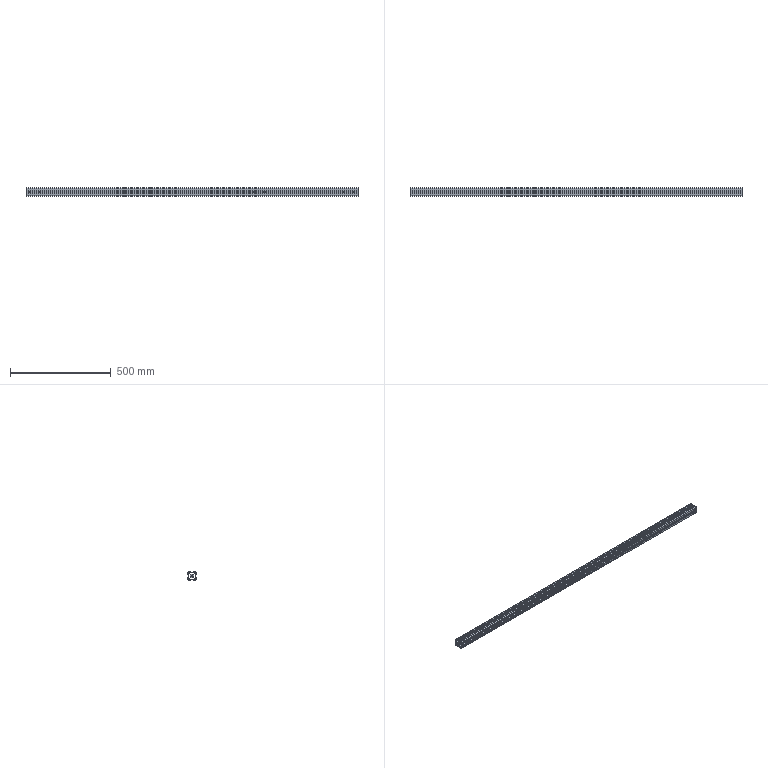Part | 1 solid | 128 faces | box 1650 x 40 x 40 mm | volume 948036 mm3 | plane 94 | cylinder 34 | commonest cylinder face diameters 6.8 x14 8.2 x12 5 x4 9 x4